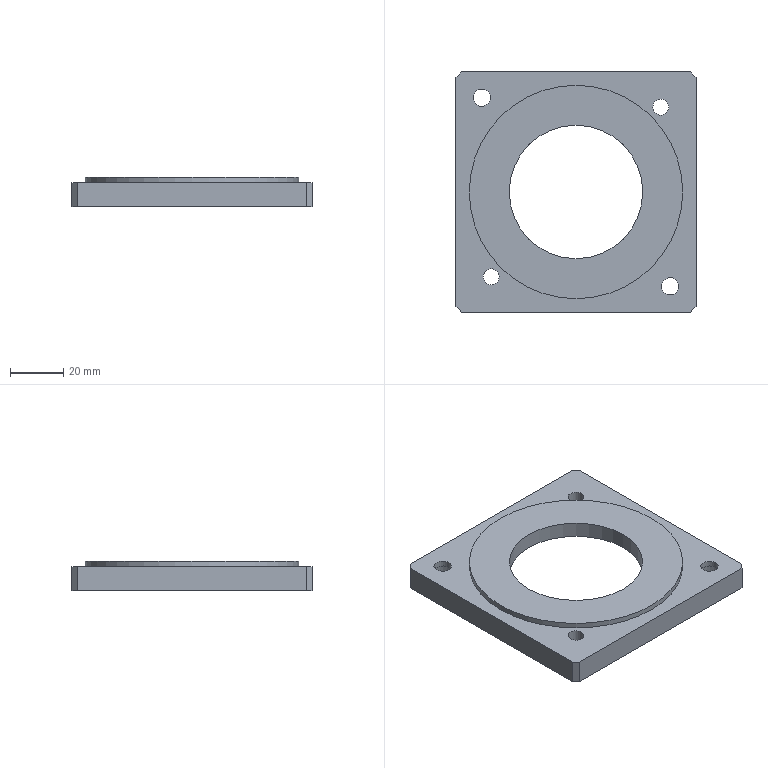NC program | NX | posted with a generic post | part box 90 x 90 x 11 mm
Lines 1756 to 1862 of 1862:
(ZLEVEL_PROFILE_COPY_1_COPY_COPY_COPY_COPY_2_COPY , TOOL : D6A45)
N3474 T07 M6
N3476 G54
N3478 G17 G0 G90 X-22.817 Y1.053 S7000 M3
N3480 G43 Z30. H7
N3482 Z-1.
N3484 G94 G1 X-23.741 Y0.52 F1000.
N3486 G3 X-24.041 Y0. R0.6
N3488 X0. Y-24.041 R24.041
N3490 X-24.041 Y0. R-24.041
N3492 X-23.741 Y-0.52 R0.6
N3494 G1 X-22.817 Y-1.053
N3496 G0 Z30.
N3498 X-42.146 Y-1.032
N3500 Z-1.
N3502 G1 X-41.259 Y-0.52
N3504 G3 X-40.959 Y0. R0.6
N3506 G2 X0. Y40.959 R40.959
N3508 X-40.959 Y0. R-40.959
N3510 G3 X-41.259 Y0.52 R0.6
N3512 G1 X-42.146 Y1.032
N3514 G0 Z30.
(ZLEVEL_PROFILE_COPY_1_COPY_COPY_COPY_COPY_2_COPY_COPY , TOOL : D6A45)
N3516 X-31.413 Y-31.083
N3518 Z-3.
N3520 G1 X-30.941 Y-30.229
N3522 G3 X-31.385 Y-29.825 R0.6
N3524 X-29.825 Y-31.385 R-2.041
N3526 X-30.229 Y-30.941 R0.6
N3528 G1 X-31.083 Y-31.413
N3530 G0 Z30.
N3532 X31.42 Y31.08
N3534 Z-3.
N3536 G1 X30.955 Y30.221
N3538 G3 X31.403 Y29.821 R0.6
N3540 X29.824 Y31.39 R-2.041
N3542 X30.227 Y30.945 R0.6
N3544 G1 X31.082 Y31.415
N3546 G0 Z30.
N3548 X36.411 Y-35.631
N3550 Z-3.
N3552 G1 X37.347 Y-35.875
N3554 G3 X37.647 Y-35.355 R0.6
N3556 X35.355 Y-33.064 R2.291
N3558 X37.647 Y-35.355 R-2.291
N3560 X37.347 Y-34.836 R0.6
N3562 G1 X36.411 Y-35.08
N3564 G0 Z30.
N3566 X-35.08 Y36.411
N3568 Z-3.
N3570 G1 X-34.836 Y37.347
N3572 G3 X-35.355 Y37.647 R0.6
N3574 X-37.647 Y35.355 R2.291
N3576 X-35.355 Y37.647 R-2.291
N3578 X-35.875 Y37.347 R0.6
N3580 G1 X-35.631 Y36.411
N3582 G0 Z30.
N3584 X-43.911 Y46.955
N3586 Z-3.
N3588 G1 X-43.509 Y46.259
N3590 G3 X-42.99 Y45.959 R0.6
N3592 G1 X42.99
N3594 G2 X43.685 Y45.67 R0.984
N3596 G1 X45.67 Y43.685
N3598 G2 X45.959 Y42.99 R0.984
N3600 G1 Y-42.99
N3602 G2 X45.67 Y-43.685 R0.984
N3604 G1 X43.685 Y-45.67
N3606 G2 X42.99 Y-45.959 R0.984
N3608 G1 X-42.99
N3610 G2 X-43.685 Y-45.67 R0.984
N3612 G1 X-45.67 Y-43.685
N3614 G2 X-45.959 Y-42.99 R0.984
N3616 G1 Y42.99
N3618 G2 X-45.67 Y43.685 R0.984
N3620 G1 X-43.685 Y45.67
N3622 G2 X-42.99 Y45.959 R0.984
N3624 G3 X-42.47 Y46.259 R0.6
N3626 G1 X-41.95 Y47.159
N3628 G0 Z30.
N3630 M5
(刀补10 , TOOL : D10)
N3632 T10 M6
N3634 G54
N3636 G17 G0 G90 X-46.587 Y-1.101 S9500 M3
N3638 G43 Z30. H10
N3640 Z-0.5
N3642 G94 G1 Z-2. F1250.
N3644 G41 X-46.487 D10
N3646 X-45.826 Y-0.985
N3648 G3 X-45. Y0. R1.
N3650 G2 X0. Y45. R45.
N3652 X-45. Y0. R-45.
N3654 G3 X-45.826 Y0.985 R1.
N3656 G1 X-46.487 Y1.101
N3658 G40
N3660 X-46.587
N3662 Z-0.5
N3664 G0 Z30.
N3666 M5
N3668 M2